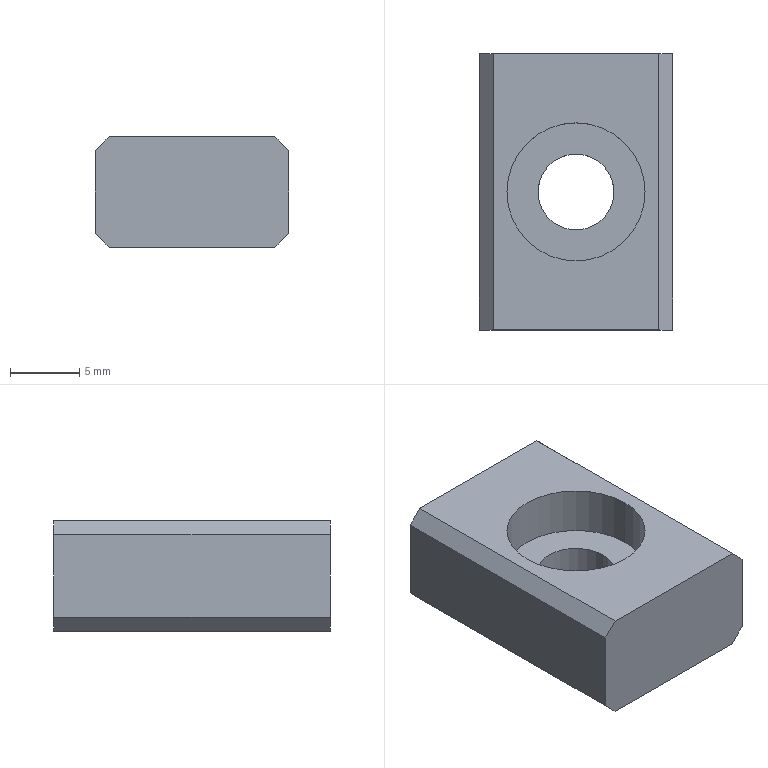Part | SolidWorks | features Cut 2, Chamfer 1, Extrusion 1 | 1 solid | 15 faces | box 14 x 20 x 8 mm | volume 1818 mm3 | plane 11 | cylinder 4 | commonest cylinder face diameters 5.5 x2 10 x2
STEP:
#1=CARTESIAN_POINT('',(-9.75,10.,-8.));
#2=VERTEX_POINT('',#1);
#3=CARTESIAN_POINT('',(-4.25,10.,-8.));
#4=VERTEX_POINT('',#3);
#5=CARTESIAN_POINT('',(-7.,10.,-8.));
#6=DIRECTION('',(0.,0.,1.));
#7=DIRECTION('',(1.,0.,0.));
#8=AXIS2_PLACEMENT_3D('',#5,#6,#7);
#9=CIRCLE('',#8,2.75);
#10=EDGE_CURVE('',#2,#4,#9,.T.);
#11=ORIENTED_EDGE('',*,*,#10,.F.);
#12=CARTESIAN_POINT('',(-9.75,10.,-3.5));
#13=VERTEX_POINT('',#12);
#14=CARTESIAN_POINT('',(-9.75,10.,-8.));
#15=DIRECTION('',(0.,0.,1.));
#16=VECTOR('',#15,1000.);
#17=LINE('',#14,#16);
#18=EDGE_CURVE('',#2,#13,#17,.T.);
#19=ORIENTED_EDGE('',*,*,#18,.T.);
#20=CARTESIAN_POINT('',(-4.25,10.,-3.5));
#21=VERTEX_POINT('',#20);
#22=CARTESIAN_POINT('',(-7.,10.,-3.5));
#23=DIRECTION('',(0.,0.,1.));
#24=DIRECTION('',(1.,0.,0.));
#25=AXIS2_PLACEMENT_3D('',#22,#23,#24);
#26=CIRCLE('',#25,2.75);
#27=EDGE_CURVE('',#13,#21,#26,.T.);
#28=ORIENTED_EDGE('',*,*,#27,.T.);
#29=CARTESIAN_POINT('',(-4.25,10.,-8.));
#30=DIRECTION('',(0.,0.,1.));
#31=VECTOR('',#30,1000.);
#32=LINE('',#29,#31);
#33=EDGE_CURVE('',#4,#21,#32,.T.);
#34=ORIENTED_EDGE('',*,*,#33,.F.);
#35=EDGE_LOOP('',(#11,#19,#28,#34));
#36=FACE_OUTER_BOUND('',#35,.T.);
#37=CARTESIAN_POINT('',(-7.,10.,-8.));
#38=DIRECTION('',(0.,0.,1.));
#39=DIRECTION('',(1.,0.,0.));
#40=AXIS2_PLACEMENT_3D('',#37,#38,#39);
#41=CYLINDRICAL_SURFACE('',#40,2.75);
#42=ADVANCED_FACE('',(#36),#41,.F.);
#43=CARTESIAN_POINT('',(-12.,10.,-3.5));
#44=VERTEX_POINT('',#43);
#45=CARTESIAN_POINT('',(-2.,10.,-3.5));
#46=VERTEX_POINT('',#45);
#47=CARTESIAN_POINT('',(-7.,10.,-3.5));
#48=DIRECTION('',(0.,0.,1.));
#49=DIRECTION('',(1.,0.,0.));
#50=AXIS2_PLACEMENT_3D('',#47,#48,#49);
#51=CIRCLE('',#50,5.);
#52=EDGE_CURVE('',#44,#46,#51,.T.);
#53=ORIENTED_EDGE('',*,*,#52,.F.);
#54=CARTESIAN_POINT('',(-12.,10.,0.));
#55=VERTEX_POINT('',#54);
#56=CARTESIAN_POINT('',(-12.,10.,-3.5));
#57=DIRECTION('',(0.,0.,1.));
#58=VECTOR('',#57,1000.);
#59=LINE('',#56,#58);
#60=EDGE_CURVE('',#44,#55,#59,.T.);
#61=ORIENTED_EDGE('',*,*,#60,.T.);
#62=CARTESIAN_POINT('',(-2.,10.,0.));
#63=VERTEX_POINT('',#62);
#64=CARTESIAN_POINT('',(-7.,10.,0.));
#65=DIRECTION('',(0.,0.,1.));
#66=DIRECTION('',(1.,0.,0.));
#67=AXIS2_PLACEMENT_3D('',#64,#65,#66);
#68=CIRCLE('',#67,5.);
#69=EDGE_CURVE('',#55,#63,#68,.T.);
#70=ORIENTED_EDGE('',*,*,#69,.T.);
#71=CARTESIAN_POINT('',(-2.,10.,-3.5));
#72=DIRECTION('',(0.,0.,1.));
#73=VECTOR('',#72,1000.);
#74=LINE('',#71,#73);
#75=EDGE_CURVE('',#46,#63,#74,.T.);
#76=ORIENTED_EDGE('',*,*,#75,.F.);
#77=EDGE_LOOP('',(#53,#61,#70,#76));
#78=FACE_OUTER_BOUND('',#77,.T.);
#79=CARTESIAN_POINT('',(-7.,10.,-3.5));
#80=DIRECTION('',(0.,0.,1.));
#81=DIRECTION('',(1.,0.,0.));
#82=AXIS2_PLACEMENT_3D('',#79,#80,#81);
#83=CYLINDRICAL_SURFACE('',#82,5.);
#84=ADVANCED_FACE('',(#78),#83,.F.);
#85=CARTESIAN_POINT('',(0.,20.,-7.));
#86=VERTEX_POINT('',#85);
#87=CARTESIAN_POINT('',(0.,20.,-1.));
#88=VERTEX_POINT('',#87);
#89=CARTESIAN_POINT('',(0.,20.,-8.));
#90=DIRECTION('',(0.,0.,1.));
#91=VECTOR('',#90,1000.);
#92=LINE('',#89,#91);
#93=EDGE_CURVE('',#86,#88,#92,.T.);
#94=ORIENTED_EDGE('',*,*,#93,.T.);
#95=CARTESIAN_POINT('',(0.,0.,-1.));
#96=VERTEX_POINT('',#95);
#97=CARTESIAN_POINT('',(0.,0.,-1.));
#98=DIRECTION('',(0.,-1.,0.));
#99=VECTOR('',#98,1000.);
#100=LINE('',#97,#99);
#101=EDGE_CURVE('',#88,#96,#100,.T.);
#102=ORIENTED_EDGE('',*,*,#101,.T.);
#103=CARTESIAN_POINT('',(0.,0.,-7.));
#104=VERTEX_POINT('',#103);
#105=CARTESIAN_POINT('',(0.,0.,-8.));
#106=DIRECTION('',(0.,0.,1.));
#107=VECTOR('',#106,1000.);
#108=LINE('',#105,#107);
#109=EDGE_CURVE('',#104,#96,#108,.T.);
#110=ORIENTED_EDGE('',*,*,#109,.F.);
#111=CARTESIAN_POINT('',(0.,20.,-7.));
#112=DIRECTION('',(0.,1.,0.));
#113=VECTOR('',#112,1000.);
#114=LINE('',#111,#113);
#115=EDGE_CURVE('',#104,#86,#114,.T.);
#116=ORIENTED_EDGE('',*,*,#115,.T.);
#117=EDGE_LOOP('',(#94,#102,#110,#116));
#118=FACE_OUTER_BOUND('',#117,.T.);
#119=CARTESIAN_POINT('',(0.,0.,-8.));
#120=DIRECTION('',(1.,0.,0.));
#121=DIRECTION('',(0.,0.,-1.));
#122=AXIS2_PLACEMENT_3D('',#119,#120,#121);
#123=PLANE('',#122);
#124=ADVANCED_FACE('',(#118),#123,.T.);
#125=CARTESIAN_POINT('',(-13.,0.,0.));
#126=VERTEX_POINT('',#125);
#127=CARTESIAN_POINT('',(-1.,0.,0.));
#128=VERTEX_POINT('',#127);
#129=CARTESIAN_POINT('',(0.,0.,0.));
#130=DIRECTION('',(1.,0.,0.));
#131=VECTOR('',#130,1000.);
#132=LINE('',#129,#131);
#133=EDGE_CURVE('',#126,#128,#132,.T.);
#134=ORIENTED_EDGE('',*,*,#133,.F.);
#135=CARTESIAN_POINT('',(-14.,0.,-1.));
#136=VERTEX_POINT('',#135);
#137=CARTESIAN_POINT('',(-10.5,0.,2.5));
#138=DIRECTION('',(-0.7071,0.,-0.7071));
#139=VECTOR('',#138,1000.);
#140=LINE('',#137,#139);
#141=EDGE_CURVE('',#126,#136,#140,.T.);
#142=ORIENTED_EDGE('',*,*,#141,.T.);
#143=CARTESIAN_POINT('',(-14.,0.,-7.));
#144=VERTEX_POINT('',#143);
#145=CARTESIAN_POINT('',(-14.,0.,-8.));
#146=DIRECTION('',(0.,0.,1.));
#147=VECTOR('',#146,1000.);
#148=LINE('',#145,#147);
#149=EDGE_CURVE('',#144,#136,#148,.T.);
#150=ORIENTED_EDGE('',*,*,#149,.F.);
#151=CARTESIAN_POINT('',(-13.,0.,-8.));
#152=VERTEX_POINT('',#151);
#153=CARTESIAN_POINT('',(-6.5,0.,-14.5));
#154=DIRECTION('',(0.7071,0.,-0.7071));
#155=VECTOR('',#154,1000.);
#156=LINE('',#153,#155);
#157=EDGE_CURVE('',#144,#152,#156,.T.);
#158=ORIENTED_EDGE('',*,*,#157,.T.);
#159=CARTESIAN_POINT('',(-1.,0.,-8.));
#160=VERTEX_POINT('',#159);
#161=CARTESIAN_POINT('',(0.,0.,-8.));
#162=DIRECTION('',(1.,0.,0.));
#163=VECTOR('',#162,1000.);
#164=LINE('',#161,#163);
#165=EDGE_CURVE('',#152,#160,#164,.T.);
#166=ORIENTED_EDGE('',*,*,#165,.T.);
#167=CARTESIAN_POINT('',(-0.5,0.,-7.5));
#168=DIRECTION('',(0.7071,0.,0.7071));
#169=VECTOR('',#168,1000.);
#170=LINE('',#167,#169);
#171=EDGE_CURVE('',#160,#104,#170,.T.);
#172=ORIENTED_EDGE('',*,*,#171,.T.);
#173=ORIENTED_EDGE('',*,*,#109,.T.);
#174=CARTESIAN_POINT('',(3.5,0.,-4.5));
#175=DIRECTION('',(-0.7071,0.,0.7071));
#176=VECTOR('',#175,1000.);
#177=LINE('',#174,#176);
#178=EDGE_CURVE('',#96,#128,#177,.T.);
#179=ORIENTED_EDGE('',*,*,#178,.T.);
#180=EDGE_LOOP('',(#134,#142,#150,#158,#166,#172,#173,#179));
#181=FACE_OUTER_BOUND('',#180,.T.);
#182=CARTESIAN_POINT('',(0.,0.,-8.));
#183=DIRECTION('',(0.,-1.,0.));
#184=DIRECTION('',(1.,0.,0.));
#185=AXIS2_PLACEMENT_3D('',#182,#183,#184);
#186=PLANE('',#185);
#187=ADVANCED_FACE('',(#181),#186,.T.);
#188=ORIENTED_EDGE('',*,*,#149,.T.);
#189=CARTESIAN_POINT('',(-14.,20.,-1.));
#190=VERTEX_POINT('',#189);
#191=CARTESIAN_POINT('',(-14.,0.,-1.));
#192=DIRECTION('',(0.,1.,0.));
#193=VECTOR('',#192,1000.);
#194=LINE('',#191,#193);
#195=EDGE_CURVE('',#136,#190,#194,.T.);
#196=ORIENTED_EDGE('',*,*,#195,.T.);
#197=CARTESIAN_POINT('',(-14.,20.,-7.));
#198=VERTEX_POINT('',#197);
#199=CARTESIAN_POINT('',(-14.,20.,-8.));
#200=DIRECTION('',(0.,0.,1.));
#201=VECTOR('',#200,1000.);
#202=LINE('',#199,#201);
#203=EDGE_CURVE('',#198,#190,#202,.T.);
#204=ORIENTED_EDGE('',*,*,#203,.F.);
#205=CARTESIAN_POINT('',(-14.,0.,-7.));
#206=DIRECTION('',(0.,-1.,0.));
#207=VECTOR('',#206,1000.);
#208=LINE('',#205,#207);
#209=EDGE_CURVE('',#198,#144,#208,.T.);
#210=ORIENTED_EDGE('',*,*,#209,.T.);
#211=EDGE_LOOP('',(#188,#196,#204,#210));
#212=FACE_OUTER_BOUND('',#211,.T.);
#213=CARTESIAN_POINT('',(-14.,0.,-8.));
#214=DIRECTION('',(-1.,0.,0.));
#215=DIRECTION('',(0.,0.,1.));
#216=AXIS2_PLACEMENT_3D('',#213,#214,#215);
#217=PLANE('',#216);
#218=ADVANCED_FACE('',(#212),#217,.T.);
#219=ORIENTED_EDGE('',*,*,#203,.T.);
#220=CARTESIAN_POINT('',(-13.,20.,0.));
#221=VERTEX_POINT('',#220);
#222=CARTESIAN_POINT('',(-10.5,20.,2.5));
#223=DIRECTION('',(0.7071,0.,0.7071));
#224=VECTOR('',#223,1000.);
#225=LINE('',#222,#224);
#226=EDGE_CURVE('',#190,#221,#225,.T.);
#227=ORIENTED_EDGE('',*,*,#226,.T.);
#228=CARTESIAN_POINT('',(-1.,20.,0.));
#229=VERTEX_POINT('',#228);
#230=CARTESIAN_POINT('',(0.,20.,0.));
#231=DIRECTION('',(-1.,0.,0.));
#232=VECTOR('',#231,1000.);
#233=LINE('',#230,#232);
#234=EDGE_CURVE('',#229,#221,#233,.T.);
#235=ORIENTED_EDGE('',*,*,#234,.F.);
#236=CARTESIAN_POINT('',(3.5,20.,-4.5));
#237=DIRECTION('',(0.7071,0.,-0.7071));
#238=VECTOR('',#237,1000.);
#239=LINE('',#236,#238);
#240=EDGE_CURVE('',#229,#88,#239,.T.);
#241=ORIENTED_EDGE('',*,*,#240,.T.);
#242=ORIENTED_EDGE('',*,*,#93,.F.);
#243=CARTESIAN_POINT('',(-1.,20.,-8.));
#244=VERTEX_POINT('',#243);
#245=CARTESIAN_POINT('',(-0.5,20.,-7.5));
#246=DIRECTION('',(-0.7071,0.,-0.7071));
#247=VECTOR('',#246,1000.);
#248=LINE('',#245,#247);
#249=EDGE_CURVE('',#86,#244,#248,.T.);
#250=ORIENTED_EDGE('',*,*,#249,.T.);
#251=CARTESIAN_POINT('',(-13.,20.,-8.));
#252=VERTEX_POINT('',#251);
#253=CARTESIAN_POINT('',(0.,20.,-8.));
#254=DIRECTION('',(-1.,0.,0.));
#255=VECTOR('',#254,1000.);
#256=LINE('',#253,#255);
#257=EDGE_CURVE('',#244,#252,#256,.T.);
#258=ORIENTED_EDGE('',*,*,#257,.T.);
#259=CARTESIAN_POINT('',(-6.5,20.,-14.5));
#260=DIRECTION('',(-0.7071,0.,0.7071));
#261=VECTOR('',#260,1000.);
#262=LINE('',#259,#261);
#263=EDGE_CURVE('',#252,#198,#262,.T.);
#264=ORIENTED_EDGE('',*,*,#263,.T.);
#265=EDGE_LOOP('',(#219,#227,#235,#241,#242,#250,#258,#264));
#266=FACE_OUTER_BOUND('',#265,.T.);
#267=CARTESIAN_POINT('',(0.,20.,-8.));
#268=DIRECTION('',(0.,1.,0.));
#269=DIRECTION('',(0.,0.,1.));
#270=AXIS2_PLACEMENT_3D('',#267,#268,#269);
#271=PLANE('',#270);
#272=ADVANCED_FACE('',(#266),#271,.T.);
#273=CARTESIAN_POINT('',(-7.,10.,-8.));
#274=DIRECTION('',(0.,0.,1.));
#275=DIRECTION('',(1.,0.,0.));
#276=AXIS2_PLACEMENT_3D('',#273,#274,#275);
#277=CIRCLE('',#276,2.75);
#278=EDGE_CURVE('',#4,#2,#277,.T.);
#279=ORIENTED_EDGE('',*,*,#278,.T.);
#280=ORIENTED_EDGE('',*,*,#10,.T.);
#281=EDGE_LOOP('',(#279,#280));
#282=FACE_BOUND('',#281,.T.);
#283=ORIENTED_EDGE('',*,*,#165,.F.);
#284=CARTESIAN_POINT('',(-13.,20.,-8.));
#285=DIRECTION('',(0.,1.,0.));
#286=VECTOR('',#285,1000.);
#287=LINE('',#284,#286);
#288=EDGE_CURVE('',#152,#252,#287,.T.);
#289=ORIENTED_EDGE('',*,*,#288,.T.);
#290=ORIENTED_EDGE('',*,*,#257,.F.);
#291=CARTESIAN_POINT('',(-1.,0.,-8.));
#292=DIRECTION('',(0.,-1.,0.));
#293=VECTOR('',#292,1000.);
#294=LINE('',#291,#293);
#295=EDGE_CURVE('',#244,#160,#294,.T.);
#296=ORIENTED_EDGE('',*,*,#295,.T.);
#297=EDGE_LOOP('',(#283,#289,#290,#296));
#298=FACE_OUTER_BOUND('',#297,.T.);
#299=CARTESIAN_POINT('',(0.,20.,-8.));
#300=DIRECTION('',(0.,0.,1.));
#301=DIRECTION('',(1.,0.,0.));
#302=AXIS2_PLACEMENT_3D('',#299,#300,#301);
#303=PLANE('',#302);
#304=ADVANCED_FACE('',(#282,#298),#303,.F.);
#305=CARTESIAN_POINT('',(-7.,10.,0.));
#306=DIRECTION('',(0.,0.,1.));
#307=DIRECTION('',(1.,0.,0.));
#308=AXIS2_PLACEMENT_3D('',#305,#306,#307);
#309=CIRCLE('',#308,5.);
#310=EDGE_CURVE('',#63,#55,#309,.T.);
#311=ORIENTED_EDGE('',*,*,#310,.F.);
#312=ORIENTED_EDGE('',*,*,#69,.F.);
#313=EDGE_LOOP('',(#311,#312));
#314=FACE_BOUND('',#313,.T.);
#315=ORIENTED_EDGE('',*,*,#234,.T.);
#316=CARTESIAN_POINT('',(-13.,20.,0.));
#317=DIRECTION('',(0.,-1.,0.));
#318=VECTOR('',#317,1000.);
#319=LINE('',#316,#318);
#320=EDGE_CURVE('',#221,#126,#319,.T.);
#321=ORIENTED_EDGE('',*,*,#320,.T.);
#322=ORIENTED_EDGE('',*,*,#133,.T.);
#323=CARTESIAN_POINT('',(-1.,20.,0.));
#324=DIRECTION('',(0.,1.,0.));
#325=VECTOR('',#324,1000.);
#326=LINE('',#323,#325);
#327=EDGE_CURVE('',#128,#229,#326,.T.);
#328=ORIENTED_EDGE('',*,*,#327,.T.);
#329=EDGE_LOOP('',(#315,#321,#322,#328));
#330=FACE_OUTER_BOUND('',#329,.T.);
#331=CARTESIAN_POINT('',(0.,20.,0.));
#332=DIRECTION('',(0.,0.,1.));
#333=DIRECTION('',(1.,0.,0.));
#334=AXIS2_PLACEMENT_3D('',#331,#332,#333);
#335=PLANE('',#334);
#336=ADVANCED_FACE('',(#314,#330),#335,.T.);
#337=ORIENTED_EDGE('',*,*,#60,.F.);
#338=CARTESIAN_POINT('',(-7.,10.,-3.5));
#339=DIRECTION('',(0.,0.,1.));
#340=DIRECTION('',(1.,0.,0.));
#341=AXIS2_PLACEMENT_3D('',#338,#339,#340);
#342=CIRCLE('',#341,5.);
#343=EDGE_CURVE('',#46,#44,#342,.T.);
#344=ORIENTED_EDGE('',*,*,#343,.F.);
#345=ORIENTED_EDGE('',*,*,#75,.T.);
#346=ORIENTED_EDGE('',*,*,#310,.T.);
#347=EDGE_LOOP('',(#337,#344,#345,#346));
#348=FACE_OUTER_BOUND('',#347,.T.);
#349=CARTESIAN_POINT('',(-7.,10.,-3.5));
#350=DIRECTION('',(0.,0.,1.));
#351=DIRECTION('',(1.,0.,0.));
#352=AXIS2_PLACEMENT_3D('',#349,#350,#351);
#353=CYLINDRICAL_SURFACE('',#352,5.);
#354=ADVANCED_FACE('',(#348),#353,.F.);
#355=CARTESIAN_POINT('',(-7.,10.,-3.5));
#356=DIRECTION('',(0.,0.,1.));
#357=DIRECTION('',(1.,0.,0.));
#358=AXIS2_PLACEMENT_3D('',#355,#356,#357);
#359=CIRCLE('',#358,2.75);
#360=EDGE_CURVE('',#21,#13,#359,.T.);
#361=ORIENTED_EDGE('',*,*,#360,.F.);
#362=ORIENTED_EDGE('',*,*,#27,.F.);
#363=EDGE_LOOP('',(#361,#362));
#364=FACE_BOUND('',#363,.T.);
#365=ORIENTED_EDGE('',*,*,#343,.T.);
#366=ORIENTED_EDGE('',*,*,#52,.T.);
#367=EDGE_LOOP('',(#365,#366));
#368=FACE_OUTER_BOUND('',#367,.T.);
#369=CARTESIAN_POINT('',(-7.,10.,-3.5));
#370=DIRECTION('',(0.,0.,1.));
#371=DIRECTION('',(1.,0.,0.));
#372=AXIS2_PLACEMENT_3D('',#369,#370,#371);
#373=PLANE('',#372);
#374=ADVANCED_FACE('',(#364,#368),#373,.T.);
#375=ORIENTED_EDGE('',*,*,#18,.F.);
#376=ORIENTED_EDGE('',*,*,#278,.F.);
#377=ORIENTED_EDGE('',*,*,#33,.T.);
#378=ORIENTED_EDGE('',*,*,#360,.T.);
#379=EDGE_LOOP('',(#375,#376,#377,#378));
#380=FACE_OUTER_BOUND('',#379,.T.);
#381=CARTESIAN_POINT('',(-7.,10.,-8.));
#382=DIRECTION('',(0.,0.,1.));
#383=DIRECTION('',(1.,0.,0.));
#384=AXIS2_PLACEMENT_3D('',#381,#382,#383);
#385=CYLINDRICAL_SURFACE('',#384,2.75);
#386=ADVANCED_FACE('',(#380),#385,.F.);
#387=ORIENTED_EDGE('',*,*,#226,.F.);
#388=ORIENTED_EDGE('',*,*,#195,.F.);
#389=ORIENTED_EDGE('',*,*,#141,.F.);
#390=ORIENTED_EDGE('',*,*,#320,.F.);
#391=EDGE_LOOP('',(#387,#388,#389,#390));
#392=FACE_OUTER_BOUND('',#391,.T.);
#393=CARTESIAN_POINT('',(-13.,20.,0.));
#394=DIRECTION('',(0.7071,0.,-0.7071));
#395=DIRECTION('',(-0.7071,0.,-0.7071));
#396=AXIS2_PLACEMENT_3D('',#393,#394,#395);
#397=PLANE('',#396);
#398=ADVANCED_FACE('',(#392),#397,.F.);
#399=ORIENTED_EDGE('',*,*,#178,.F.);
#400=ORIENTED_EDGE('',*,*,#101,.F.);
#401=ORIENTED_EDGE('',*,*,#240,.F.);
#402=ORIENTED_EDGE('',*,*,#327,.F.);
#403=EDGE_LOOP('',(#399,#400,#401,#402));
#404=FACE_OUTER_BOUND('',#403,.T.);
#405=CARTESIAN_POINT('',(-1.,20.,0.));
#406=DIRECTION('',(-0.7071,0.,-0.7071));
#407=DIRECTION('',(-0.7071,0.,0.7071));
#408=AXIS2_PLACEMENT_3D('',#405,#406,#407);
#409=PLANE('',#408);
#410=ADVANCED_FACE('',(#404),#409,.F.);
#411=ORIENTED_EDGE('',*,*,#263,.F.);
#412=ORIENTED_EDGE('',*,*,#288,.F.);
#413=ORIENTED_EDGE('',*,*,#157,.F.);
#414=ORIENTED_EDGE('',*,*,#209,.F.);
#415=EDGE_LOOP('',(#411,#412,#413,#414));
#416=FACE_OUTER_BOUND('',#415,.T.);
#417=CARTESIAN_POINT('',(-14.,0.,-7.));
#418=DIRECTION('',(-0.7071,0.,-0.7071));
#419=DIRECTION('',(-0.7071,0.,0.7071));
#420=AXIS2_PLACEMENT_3D('',#417,#418,#419);
#421=PLANE('',#420);
#422=ADVANCED_FACE('',(#416),#421,.T.);
#423=ORIENTED_EDGE('',*,*,#171,.F.);
#424=ORIENTED_EDGE('',*,*,#295,.F.);
#425=ORIENTED_EDGE('',*,*,#249,.F.);
#426=ORIENTED_EDGE('',*,*,#115,.F.);
#427=EDGE_LOOP('',(#423,#424,#425,#426));
#428=FACE_OUTER_BOUND('',#427,.T.);
#429=CARTESIAN_POINT('',(0.,0.,-7.));
#430=DIRECTION('',(0.7071,0.,-0.7071));
#431=DIRECTION('',(-0.7071,0.,-0.7071));
#432=AXIS2_PLACEMENT_3D('',#429,#430,#431);
#433=PLANE('',#432);
#434=ADVANCED_FACE('',(#428),#433,.T.);
#435=CLOSED_SHELL('',(#42,#84,#124,#187,#218,#272,#304,#336,#354,#374,#386,#398,#410,#422,#434));
#436=MANIFOLD_SOLID_BREP('',#435);
#437=CARTESIAN_POINT('',(0.,0.,0.));
#438=DIRECTION('',(0.,0.,1.));
#439=DIRECTION('',(1.,0.,0.));
#440=AXIS2_PLACEMENT_3D('',#437,#438,#439);
#441=(LENGTH_UNIT()NAMED_UNIT(*)SI_UNIT(.MILLI.,.METRE.));
#442=UNCERTAINTY_MEASURE_WITH_UNIT(LENGTH_MEASURE(0.00001),#441,'','');
#443=(NAMED_UNIT(*)PLANE_ANGLE_UNIT()SI_UNIT($,.RADIAN.));
#444=(NAMED_UNIT(*)SI_UNIT($,.STERADIAN.)SOLID_ANGLE_UNIT());
#445=(GEOMETRIC_REPRESENTATION_CONTEXT(3)GLOBAL_UNCERTAINTY_ASSIGNED_CONTEXT((#442))GLOBAL_UNIT_ASSIGNED_CONTEXT((#441,#443,#444))REPRESENTATION_CONTEXT('',''));
#446=ADVANCED_BREP_SHAPE_REPRESENTATION('',(#436,#440),#445);